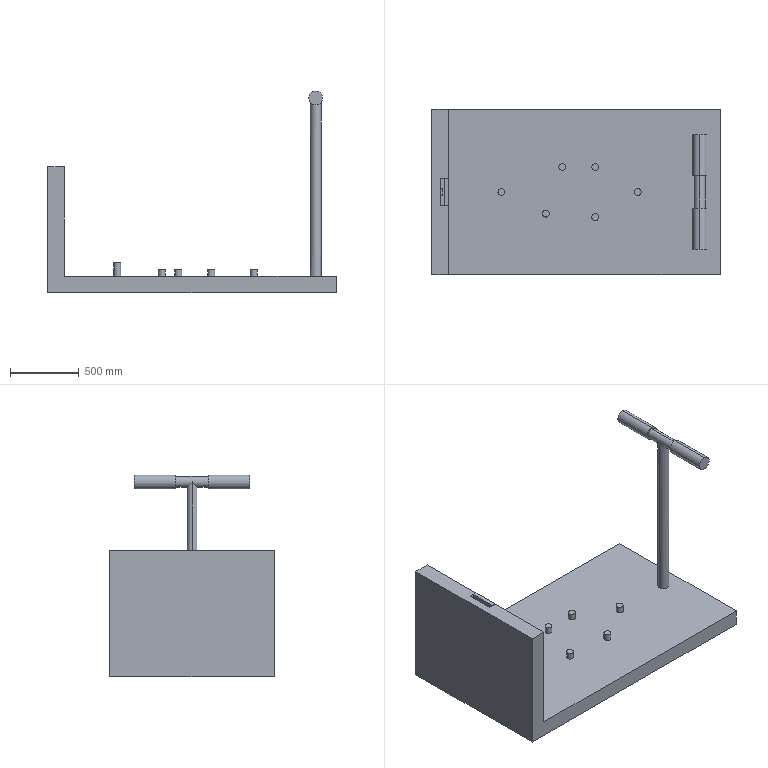Part | SolidWorks | features ICE 12, Extrusion 1, MirrorPattern 1 | 2 solids | 52 faces | box 2100 x 1200 x 1470 mm | volume 421779830 mm3 | plane 32 | cylinder 20 | commonest cylinder face diameters 50 x12 80 x4 100 x4
STEP:
#1=CARTESIAN_POINT('',(531.866,-600.,220.));
#2=VERTEX_POINT('',#1);
#3=CARTESIAN_POINT('',(481.866,-600.,220.));
#4=VERTEX_POINT('',#3);
#5=CARTESIAN_POINT('',(506.866,-600.,220.));
#6=DIRECTION('',(0.,0.,1.));
#7=DIRECTION('',(1.,0.,0.));
#8=AXIS2_PLACEMENT_3D('',#5,#6,#7);
#9=CIRCLE('',#8,25.);
#10=EDGE_CURVE('',#2,#4,#9,.T.);
#11=ORIENTED_EDGE('',*,*,#10,.F.);
#12=CARTESIAN_POINT('',(531.866,-600.,120.));
#13=VERTEX_POINT('',#12);
#14=CARTESIAN_POINT('',(531.866,-600.,220.));
#15=DIRECTION('',(0.,0.,-1.));
#16=VECTOR('',#15,1000.);
#17=LINE('',#14,#16);
#18=EDGE_CURVE('',#2,#13,#17,.T.);
#19=ORIENTED_EDGE('',*,*,#18,.T.);
#20=CARTESIAN_POINT('',(481.866,-600.,120.));
#21=VERTEX_POINT('',#20);
#22=CARTESIAN_POINT('',(506.866,-600.,120.));
#23=DIRECTION('',(0.,0.,1.));
#24=DIRECTION('',(1.,0.,0.));
#25=AXIS2_PLACEMENT_3D('',#22,#23,#24);
#26=CIRCLE('',#25,25.);
#27=EDGE_CURVE('',#13,#21,#26,.T.);
#28=ORIENTED_EDGE('',*,*,#27,.T.);
#29=CARTESIAN_POINT('',(481.866,-600.,220.));
#30=DIRECTION('',(0.,0.,-1.));
#31=VECTOR('',#30,1000.);
#32=LINE('',#29,#31);
#33=EDGE_CURVE('',#4,#21,#32,.T.);
#34=ORIENTED_EDGE('',*,*,#33,.F.);
#35=EDGE_LOOP('',(#11,#19,#28,#34));
#36=FACE_OUTER_BOUND('',#35,.T.);
#37=CARTESIAN_POINT('',(506.866,-600.,220.));
#38=DIRECTION('',(0.,0.,-1.));
#39=DIRECTION('',(-1.,0.,0.));
#40=AXIS2_PLACEMENT_3D('',#37,#38,#39);
#41=CYLINDRICAL_SURFACE('',#40,25.);
#42=ADVANCED_FACE('',(#36),#41,.T.);
#43=CARTESIAN_POINT('',(855.963,-756.72,170.));
#44=VERTEX_POINT('',#43);
#45=CARTESIAN_POINT('',(805.963,-756.72,170.));
#46=VERTEX_POINT('',#45);
#47=CARTESIAN_POINT('',(830.963,-756.72,170.));
#48=DIRECTION('',(0.,0.,1.));
#49=DIRECTION('',(1.,0.,0.));
#50=AXIS2_PLACEMENT_3D('',#47,#48,#49);
#51=CIRCLE('',#50,25.);
#52=EDGE_CURVE('',#44,#46,#51,.T.);
#53=ORIENTED_EDGE('',*,*,#52,.F.);
#54=CARTESIAN_POINT('',(855.963,-756.72,120.));
#55=VERTEX_POINT('',#54);
#56=CARTESIAN_POINT('',(855.963,-756.72,170.));
#57=DIRECTION('',(0.,0.,-1.));
#58=VECTOR('',#57,1000.);
#59=LINE('',#56,#58);
#60=EDGE_CURVE('',#44,#55,#59,.T.);
#61=ORIENTED_EDGE('',*,*,#60,.T.);
#62=CARTESIAN_POINT('',(805.963,-756.72,120.));
#63=VERTEX_POINT('',#62);
#64=CARTESIAN_POINT('',(830.963,-756.72,120.));
#65=DIRECTION('',(0.,0.,1.));
#66=DIRECTION('',(1.,0.,0.));
#67=AXIS2_PLACEMENT_3D('',#64,#65,#66);
#68=CIRCLE('',#67,25.);
#69=EDGE_CURVE('',#55,#63,#68,.T.);
#70=ORIENTED_EDGE('',*,*,#69,.T.);
#71=CARTESIAN_POINT('',(805.963,-756.72,170.));
#72=DIRECTION('',(0.,0.,-1.));
#73=VECTOR('',#72,1000.);
#74=LINE('',#71,#73);
#75=EDGE_CURVE('',#46,#63,#74,.T.);
#76=ORIENTED_EDGE('',*,*,#75,.F.);
#77=EDGE_LOOP('',(#53,#61,#70,#76));
#78=FACE_OUTER_BOUND('',#77,.T.);
#79=CARTESIAN_POINT('',(830.963,-756.72,170.));
#80=DIRECTION('',(0.,0.,-1.));
#81=DIRECTION('',(-1.,0.,0.));
#82=AXIS2_PLACEMENT_3D('',#79,#80,#81);
#83=CYLINDRICAL_SURFACE('',#82,25.);
#84=ADVANCED_FACE('',(#78),#83,.T.);
#85=CARTESIAN_POINT('',(975.,-416.97,170.));
#86=VERTEX_POINT('',#85);
#87=CARTESIAN_POINT('',(925.,-416.97,170.));
#88=VERTEX_POINT('',#87);
#89=CARTESIAN_POINT('',(950.,-416.97,170.));
#90=DIRECTION('',(0.,0.,1.));
#91=DIRECTION('',(1.,0.,0.));
#92=AXIS2_PLACEMENT_3D('',#89,#90,#91);
#93=CIRCLE('',#92,25.);
#94=EDGE_CURVE('',#86,#88,#93,.T.);
#95=ORIENTED_EDGE('',*,*,#94,.F.);
#96=CARTESIAN_POINT('',(975.,-416.97,120.));
#97=VERTEX_POINT('',#96);
#98=CARTESIAN_POINT('',(975.,-416.97,170.));
#99=DIRECTION('',(0.,0.,-1.));
#100=VECTOR('',#99,1000.);
#101=LINE('',#98,#100);
#102=EDGE_CURVE('',#86,#97,#101,.T.);
#103=ORIENTED_EDGE('',*,*,#102,.T.);
#104=CARTESIAN_POINT('',(925.,-416.97,120.));
#105=VERTEX_POINT('',#104);
#106=CARTESIAN_POINT('',(950.,-416.97,120.));
#107=DIRECTION('',(0.,0.,1.));
#108=DIRECTION('',(1.,0.,0.));
#109=AXIS2_PLACEMENT_3D('',#106,#107,#108);
#110=CIRCLE('',#109,25.);
#111=EDGE_CURVE('',#97,#105,#110,.T.);
#112=ORIENTED_EDGE('',*,*,#111,.T.);
#113=CARTESIAN_POINT('',(925.,-416.97,170.));
#114=DIRECTION('',(0.,0.,-1.));
#115=VECTOR('',#114,1000.);
#116=LINE('',#113,#115);
#117=EDGE_CURVE('',#88,#105,#116,.T.);
#118=ORIENTED_EDGE('',*,*,#117,.F.);
#119=EDGE_LOOP('',(#95,#103,#112,#118));
#120=FACE_OUTER_BOUND('',#119,.T.);
#121=CARTESIAN_POINT('',(950.,-416.97,170.));
#122=DIRECTION('',(0.,0.,-1.));
#123=DIRECTION('',(-1.,0.,0.));
#124=AXIS2_PLACEMENT_3D('',#121,#122,#123);
#125=CYLINDRICAL_SURFACE('',#124,25.);
#126=ADVANCED_FACE('',(#120),#125,.T.);
#127=CARTESIAN_POINT('',(1215.,-783.03,170.));
#128=VERTEX_POINT('',#127);
#129=CARTESIAN_POINT('',(1165.,-783.03,170.));
#130=VERTEX_POINT('',#129);
#131=CARTESIAN_POINT('',(1190.,-783.03,170.));
#132=DIRECTION('',(0.,0.,1.));
#133=DIRECTION('',(1.,0.,0.));
#134=AXIS2_PLACEMENT_3D('',#131,#132,#133);
#135=CIRCLE('',#134,25.);
#136=EDGE_CURVE('',#128,#130,#135,.T.);
#137=ORIENTED_EDGE('',*,*,#136,.F.);
#138=CARTESIAN_POINT('',(1215.,-783.03,120.));
#139=VERTEX_POINT('',#138);
#140=CARTESIAN_POINT('',(1215.,-783.03,170.));
#141=DIRECTION('',(0.,0.,-1.));
#142=VECTOR('',#141,1000.);
#143=LINE('',#140,#142);
#144=EDGE_CURVE('',#128,#139,#143,.T.);
#145=ORIENTED_EDGE('',*,*,#144,.T.);
#146=CARTESIAN_POINT('',(1165.,-783.03,120.));
#147=VERTEX_POINT('',#146);
#148=CARTESIAN_POINT('',(1190.,-783.03,120.));
#149=DIRECTION('',(0.,0.,1.));
#150=DIRECTION('',(1.,0.,0.));
#151=AXIS2_PLACEMENT_3D('',#148,#149,#150);
#152=CIRCLE('',#151,25.);
#153=EDGE_CURVE('',#139,#147,#152,.T.);
#154=ORIENTED_EDGE('',*,*,#153,.T.);
#155=CARTESIAN_POINT('',(1165.,-783.03,170.));
#156=DIRECTION('',(0.,0.,-1.));
#157=VECTOR('',#156,1000.);
#158=LINE('',#155,#157);
#159=EDGE_CURVE('',#130,#147,#158,.T.);
#160=ORIENTED_EDGE('',*,*,#159,.F.);
#161=EDGE_LOOP('',(#137,#145,#154,#160));
#162=FACE_OUTER_BOUND('',#161,.T.);
#163=CARTESIAN_POINT('',(1190.,-783.03,170.));
#164=DIRECTION('',(0.,0.,-1.));
#165=DIRECTION('',(-1.,0.,0.));
#166=AXIS2_PLACEMENT_3D('',#163,#164,#165);
#167=CYLINDRICAL_SURFACE('',#166,25.);
#168=ADVANCED_FACE('',(#162),#167,.T.);
#169=CARTESIAN_POINT('',(1215.,-416.97,170.));
#170=VERTEX_POINT('',#169);
#171=CARTESIAN_POINT('',(1165.,-416.97,170.));
#172=VERTEX_POINT('',#171);
#173=CARTESIAN_POINT('',(1190.,-416.97,170.));
#174=DIRECTION('',(0.,0.,1.));
#175=DIRECTION('',(1.,0.,0.));
#176=AXIS2_PLACEMENT_3D('',#173,#174,#175);
#177=CIRCLE('',#176,25.);
#178=EDGE_CURVE('',#170,#172,#177,.T.);
#179=ORIENTED_EDGE('',*,*,#178,.F.);
#180=CARTESIAN_POINT('',(1215.,-416.97,120.));
#181=VERTEX_POINT('',#180);
#182=CARTESIAN_POINT('',(1215.,-416.97,170.));
#183=DIRECTION('',(0.,0.,-1.));
#184=VECTOR('',#183,1000.);
#185=LINE('',#182,#184);
#186=EDGE_CURVE('',#170,#181,#185,.T.);
#187=ORIENTED_EDGE('',*,*,#186,.T.);
#188=CARTESIAN_POINT('',(1165.,-416.97,120.));
#189=VERTEX_POINT('',#188);
#190=CARTESIAN_POINT('',(1190.,-416.97,120.));
#191=DIRECTION('',(0.,0.,1.));
#192=DIRECTION('',(1.,0.,0.));
#193=AXIS2_PLACEMENT_3D('',#190,#191,#192);
#194=CIRCLE('',#193,25.);
#195=EDGE_CURVE('',#181,#189,#194,.T.);
#196=ORIENTED_EDGE('',*,*,#195,.T.);
#197=CARTESIAN_POINT('',(1165.,-416.97,170.));
#198=DIRECTION('',(0.,0.,-1.));
#199=VECTOR('',#198,1000.);
#200=LINE('',#197,#199);
#201=EDGE_CURVE('',#172,#189,#200,.T.);
#202=ORIENTED_EDGE('',*,*,#201,.F.);
#203=EDGE_LOOP('',(#179,#187,#196,#202));
#204=FACE_OUTER_BOUND('',#203,.T.);
#205=CARTESIAN_POINT('',(1190.,-416.97,170.));
#206=DIRECTION('',(0.,0.,-1.));
#207=DIRECTION('',(-1.,0.,0.));
#208=AXIS2_PLACEMENT_3D('',#205,#206,#207);
#209=CYLINDRICAL_SURFACE('',#208,25.);
#210=ADVANCED_FACE('',(#204),#209,.T.);
#211=CARTESIAN_POINT('',(1525.,-600.,170.));
#212=VERTEX_POINT('',#211);
#213=CARTESIAN_POINT('',(1475.,-600.,170.));
#214=VERTEX_POINT('',#213);
#215=CARTESIAN_POINT('',(1500.,-600.,170.));
#216=DIRECTION('',(0.,0.,1.));
#217=DIRECTION('',(1.,0.,0.));
#218=AXIS2_PLACEMENT_3D('',#215,#216,#217);
#219=CIRCLE('',#218,25.);
#220=EDGE_CURVE('',#212,#214,#219,.T.);
#221=ORIENTED_EDGE('',*,*,#220,.F.);
#222=CARTESIAN_POINT('',(1525.,-600.,120.));
#223=VERTEX_POINT('',#222);
#224=CARTESIAN_POINT('',(1525.,-600.,170.));
#225=DIRECTION('',(0.,0.,-1.));
#226=VECTOR('',#225,1000.);
#227=LINE('',#224,#226);
#228=EDGE_CURVE('',#212,#223,#227,.T.);
#229=ORIENTED_EDGE('',*,*,#228,.T.);
#230=CARTESIAN_POINT('',(1475.,-600.,120.));
#231=VERTEX_POINT('',#230);
#232=CARTESIAN_POINT('',(1500.,-600.,120.));
#233=DIRECTION('',(0.,0.,1.));
#234=DIRECTION('',(1.,0.,0.));
#235=AXIS2_PLACEMENT_3D('',#232,#233,#234);
#236=CIRCLE('',#235,25.);
#237=EDGE_CURVE('',#223,#231,#236,.T.);
#238=ORIENTED_EDGE('',*,*,#237,.T.);
#239=CARTESIAN_POINT('',(1475.,-600.,170.));
#240=DIRECTION('',(0.,0.,-1.));
#241=VECTOR('',#240,1000.);
#242=LINE('',#239,#241);
#243=EDGE_CURVE('',#214,#231,#242,.T.);
#244=ORIENTED_EDGE('',*,*,#243,.F.);
#245=EDGE_LOOP('',(#221,#229,#238,#244));
#246=FACE_OUTER_BOUND('',#245,.T.);
#247=CARTESIAN_POINT('',(1500.,-600.,170.));
#248=DIRECTION('',(0.,0.,-1.));
#249=DIRECTION('',(-1.,0.,0.));
#250=AXIS2_PLACEMENT_3D('',#247,#248,#249);
#251=CYLINDRICAL_SURFACE('',#250,25.);
#252=ADVANCED_FACE('',(#246),#251,.T.);
#253=CARTESIAN_POINT('',(1950.,-180.,1370.));
#254=VERTEX_POINT('',#253);
#255=CARTESIAN_POINT('',(1950.,-180.,1470.));
#256=VERTEX_POINT('',#255);
#257=CARTESIAN_POINT('',(1950.,-180.,1420.));
#258=DIRECTION('',(0.,-1.,0.));
#259=DIRECTION('',(0.,0.,-1.));
#260=AXIS2_PLACEMENT_3D('',#257,#258,#259);
#261=CIRCLE('',#260,50.);
#262=EDGE_CURVE('',#254,#256,#261,.T.);
#263=ORIENTED_EDGE('',*,*,#262,.T.);
#264=CARTESIAN_POINT('',(1950.,-480.,1470.));
#265=VERTEX_POINT('',#264);
#266=CARTESIAN_POINT('',(1950.,-180.,1470.));
#267=DIRECTION('',(0.,-1.,0.));
#268=VECTOR('',#267,1000.);
#269=LINE('',#266,#268);
#270=EDGE_CURVE('',#256,#265,#269,.T.);
#271=ORIENTED_EDGE('',*,*,#270,.T.);
#272=CARTESIAN_POINT('',(1950.,-480.,1370.));
#273=VERTEX_POINT('',#272);
#274=CARTESIAN_POINT('',(1950.,-480.,1420.));
#275=DIRECTION('',(0.,-1.,0.));
#276=DIRECTION('',(0.,0.,-1.));
#277=AXIS2_PLACEMENT_3D('',#274,#275,#276);
#278=CIRCLE('',#277,50.);
#279=EDGE_CURVE('',#273,#265,#278,.T.);
#280=ORIENTED_EDGE('',*,*,#279,.F.);
#281=CARTESIAN_POINT('',(1950.,-180.,1370.));
#282=DIRECTION('',(0.,-1.,0.));
#283=VECTOR('',#282,1000.);
#284=LINE('',#281,#283);
#285=EDGE_CURVE('',#254,#273,#284,.T.);
#286=ORIENTED_EDGE('',*,*,#285,.F.);
#287=EDGE_LOOP('',(#263,#271,#280,#286));
#288=FACE_OUTER_BOUND('',#287,.T.);
#289=CARTESIAN_POINT('',(1950.,-180.,1420.));
#290=DIRECTION('',(0.,-1.,0.));
#291=DIRECTION('',(0.,0.,-1.));
#292=AXIS2_PLACEMENT_3D('',#289,#290,#291);
#293=CYLINDRICAL_SURFACE('',#292,50.);
#294=ADVANCED_FACE('',(#288),#293,.T.);
#295=CARTESIAN_POINT('',(1950.,-1020.,1370.));
#296=VERTEX_POINT('',#295);
#297=CARTESIAN_POINT('',(1950.,-1020.,1470.));
#298=VERTEX_POINT('',#297);
#299=CARTESIAN_POINT('',(1950.,-1020.,1420.));
#300=DIRECTION('',(0.,-1.,0.));
#301=DIRECTION('',(0.,0.,-1.));
#302=AXIS2_PLACEMENT_3D('',#299,#300,#301);
#303=CIRCLE('',#302,50.);
#304=EDGE_CURVE('',#296,#298,#303,.T.);
#305=ORIENTED_EDGE('',*,*,#304,.F.);
#306=CARTESIAN_POINT('',(1950.,-720.,1370.));
#307=VERTEX_POINT('',#306);
#308=CARTESIAN_POINT('',(1950.,-1020.,1370.));
#309=DIRECTION('',(0.,1.,0.));
#310=VECTOR('',#309,1000.);
#311=LINE('',#308,#310);
#312=EDGE_CURVE('',#296,#307,#311,.T.);
#313=ORIENTED_EDGE('',*,*,#312,.T.);
#314=CARTESIAN_POINT('',(1950.,-720.,1470.));
#315=VERTEX_POINT('',#314);
#316=CARTESIAN_POINT('',(1950.,-720.,1420.));
#317=DIRECTION('',(0.,-1.,0.));
#318=DIRECTION('',(0.,0.,-1.));
#319=AXIS2_PLACEMENT_3D('',#316,#317,#318);
#320=CIRCLE('',#319,50.);
#321=EDGE_CURVE('',#307,#315,#320,.T.);
#322=ORIENTED_EDGE('',*,*,#321,.T.);
#323=CARTESIAN_POINT('',(1950.,-1020.,1470.));
#324=DIRECTION('',(0.,1.,0.));
#325=VECTOR('',#324,1000.);
#326=LINE('',#323,#325);
#327=EDGE_CURVE('',#298,#315,#326,.T.);
#328=ORIENTED_EDGE('',*,*,#327,.F.);
#329=EDGE_LOOP('',(#305,#313,#322,#328));
#330=FACE_OUTER_BOUND('',#329,.T.);
#331=CARTESIAN_POINT('',(1950.,-1020.,1420.));
#332=DIRECTION('',(0.,1.,0.));
#333=DIRECTION('',(0.,0.,1.));
#334=AXIS2_PLACEMENT_3D('',#331,#332,#333);
#335=CYLINDRICAL_SURFACE('',#334,50.);
#336=ADVANCED_FACE('',(#330),#335,.T.);
#337=CARTESIAN_POINT('',(1950.,-480.,1380.));
#338=VERTEX_POINT('',#337);
#339=CARTESIAN_POINT('',(1950.,-480.,1460.));
#340=VERTEX_POINT('',#339);
#341=CARTESIAN_POINT('',(1950.,-480.,1420.));
#342=DIRECTION('',(0.,-1.,0.));
#343=DIRECTION('',(0.,0.,-1.));
#344=AXIS2_PLACEMENT_3D('',#341,#342,#343);
#345=CIRCLE('',#344,40.);
#346=EDGE_CURVE('',#338,#340,#345,.T.);
#347=ORIENTED_EDGE('',*,*,#346,.T.);
#348=CARTESIAN_POINT('',(1950.,-720.,1460.));
#349=VERTEX_POINT('',#348);
#350=CARTESIAN_POINT('',(1950.,-480.,1460.));
#351=DIRECTION('',(0.,-1.,0.));
#352=VECTOR('',#351,1000.);
#353=LINE('',#350,#352);
#354=EDGE_CURVE('',#340,#349,#353,.T.);
#355=ORIENTED_EDGE('',*,*,#354,.T.);
#356=CARTESIAN_POINT('',(1950.,-720.,1380.));
#357=VERTEX_POINT('',#356);
#358=CARTESIAN_POINT('',(1950.,-720.,1420.));
#359=DIRECTION('',(0.,-1.,0.));
#360=DIRECTION('',(0.,0.,-1.));
#361=AXIS2_PLACEMENT_3D('',#358,#359,#360);
#362=CIRCLE('',#361,40.);
#363=EDGE_CURVE('',#357,#349,#362,.T.);
#364=ORIENTED_EDGE('',*,*,#363,.F.);
#365=CARTESIAN_POINT('',(1950.,-640.,1380.));
#366=VERTEX_POINT('',#365);
#367=CARTESIAN_POINT('',(1950.,-480.,1380.));
#368=DIRECTION('',(0.,-1.,0.));
#369=VECTOR('',#368,1000.);
#370=LINE('',#367,#369);
#371=EDGE_CURVE('',#366,#357,#370,.T.);
#372=ORIENTED_EDGE('',*,*,#371,.F.);
#373=CARTESIAN_POINT('',(1990.,-600.,1420.));
#374=VERTEX_POINT('',#373);
#375=CARTESIAN_POINT('',(1990.,-600.,1420.));
#376=CARTESIAN_POINT('',(1990.,-623.431,1396.569));
#377=CARTESIAN_POINT('',(1973.431,-640.,1380.));
#378=CARTESIAN_POINT('',(1950.,-640.,1380.));
#379=(BOUNDED_CURVE()B_SPLINE_CURVE(3,(#375,#376,#377,#378),.UNSPECIFIED.,.F.,.F.)B_SPLINE_CURVE_WITH_KNOTS((4,4),(4.712,6.283),.UNSPECIFIED.)CURVE()GEOMETRIC_REPRESENTATION_ITEM()RATIONAL_B_SPLINE_CURVE((1.,0.8047,0.8047,1.))REPRESENTATION_ITEM(''));
#380=EDGE_CURVE('',#374,#366,#379,.T.);
#381=ORIENTED_EDGE('',*,*,#380,.F.);
#382=CARTESIAN_POINT('',(1950.,-560.,1380.));
#383=VERTEX_POINT('',#382);
#384=CARTESIAN_POINT('',(1950.,-560.,1380.));
#385=CARTESIAN_POINT('',(1973.431,-560.,1380.));
#386=CARTESIAN_POINT('',(1990.,-576.569,1396.569));
#387=CARTESIAN_POINT('',(1990.,-600.,1420.));
#388=(BOUNDED_CURVE()B_SPLINE_CURVE(3,(#384,#385,#386,#387),.UNSPECIFIED.,.F.,.F.)B_SPLINE_CURVE_WITH_KNOTS((4,4),(0.,1.571),.UNSPECIFIED.)CURVE()GEOMETRIC_REPRESENTATION_ITEM()RATIONAL_B_SPLINE_CURVE((1.,0.8047,0.8047,1.))REPRESENTATION_ITEM(''));
#389=EDGE_CURVE('',#383,#374,#388,.T.);
#390=ORIENTED_EDGE('',*,*,#389,.F.);
#391=CARTESIAN_POINT('',(1950.,-480.,1380.));
#392=DIRECTION('',(0.,-1.,0.));
#393=VECTOR('',#392,1000.);
#394=LINE('',#391,#393);
#395=EDGE_CURVE('',#338,#383,#394,.T.);
#396=ORIENTED_EDGE('',*,*,#395,.F.);
#397=EDGE_LOOP('',(#347,#355,#364,#372,#381,#390,#396));
#398=FACE_OUTER_BOUND('',#397,.T.);
#399=CARTESIAN_POINT('',(1950.,-480.,1420.));
#400=DIRECTION('',(0.,-1.,0.));
#401=DIRECTION('',(0.,0.,-1.));
#402=AXIS2_PLACEMENT_3D('',#399,#400,#401);
#403=CYLINDRICAL_SURFACE('',#402,40.);
#404=ADVANCED_FACE('',(#398),#403,.T.);
#405=CARTESIAN_POINT('',(1910.,-600.,1420.));
#406=VERTEX_POINT('',#405);
#407=CARTESIAN_POINT('',(1910.,-600.,1420.));
#408=CARTESIAN_POINT('',(1910.,-576.569,1396.569));
#409=CARTESIAN_POINT('',(1926.569,-560.,1380.));
#410=CARTESIAN_POINT('',(1950.,-560.,1380.));
#411=(BOUNDED_CURVE()B_SPLINE_CURVE(3,(#407,#408,#409,#410),.UNSPECIFIED.,.F.,.F.)B_SPLINE_CURVE_WITH_KNOTS((4,4),(4.712,6.283),.UNSPECIFIED.)CURVE()GEOMETRIC_REPRESENTATION_ITEM()RATIONAL_B_SPLINE_CURVE((1.,0.8047,0.8047,1.))REPRESENTATION_ITEM(''));
#412=EDGE_CURVE('',#406,#383,#411,.T.);
#413=ORIENTED_EDGE('',*,*,#412,.T.);
#414=ORIENTED_EDGE('',*,*,#389,.T.);
#415=CARTESIAN_POINT('',(1990.,-600.,120.));
#416=VERTEX_POINT('',#415);
#417=CARTESIAN_POINT('',(1990.,-600.,1420.));
#418=DIRECTION('',(0.,0.,-1.));
#419=VECTOR('',#418,1000.);
#420=LINE('',#417,#419);
#421=EDGE_CURVE('',#374,#416,#420,.T.);
#422=ORIENTED_EDGE('',*,*,#421,.T.);
#423=CARTESIAN_POINT('',(1910.,-600.,120.));
#424=VERTEX_POINT('',#423);
#425=CARTESIAN_POINT('',(1950.,-600.,120.));
#426=DIRECTION('',(0.,0.,1.));
#427=DIRECTION('',(1.,0.,0.));
#428=AXIS2_PLACEMENT_3D('',#425,#426,#427);
#429=CIRCLE('',#428,40.);
#430=EDGE_CURVE('',#416,#424,#429,.T.);
#431=ORIENTED_EDGE('',*,*,#430,.T.);
#432=CARTESIAN_POINT('',(1910.,-600.,1420.));
#433=DIRECTION('',(0.,0.,-1.));
#434=VECTOR('',#433,1000.);
#435=LINE('',#432,#434);
#436=EDGE_CURVE('',#406,#424,#435,.T.);
#437=ORIENTED_EDGE('',*,*,#436,.F.);
#438=EDGE_LOOP('',(#413,#414,#422,#431,#437));
#439=FACE_OUTER_BOUND('',#438,.T.);
#440=CARTESIAN_POINT('',(1950.,-600.,1420.));
#441=DIRECTION('',(0.,0.,-1.));
#442=DIRECTION('',(-1.,0.,0.));
#443=AXIS2_PLACEMENT_3D('',#440,#441,#442);
#444=CYLINDRICAL_SURFACE('',#443,40.);
#445=ADVANCED_FACE('',(#439),#444,.T.);
#446=CARTESIAN_POINT('',(506.866,-600.,120.));
#447=DIRECTION('',(0.,0.,1.));
#448=DIRECTION('',(1.,0.,0.));
#449=AXIS2_PLACEMENT_3D('',#446,#447,#448);
#450=CIRCLE('',#449,25.);
#451=EDGE_CURVE('',#21,#13,#450,.T.);
#452=ORIENTED_EDGE('',*,*,#451,.F.);
#453=ORIENTED_EDGE('',*,*,#27,.F.);
#454=EDGE_LOOP('',(#452,#453));
#455=FACE_BOUND('',#454,.T.);
#456=CARTESIAN_POINT('',(830.963,-756.72,120.));
#457=DIRECTION('',(0.,0.,1.));
#458=DIRECTION('',(1.,0.,0.));
#459=AXIS2_PLACEMENT_3D('',#456,#457,#458);
#460=CIRCLE('',#459,25.);
#461=EDGE_CURVE('',#63,#55,#460,.T.);
#462=ORIENTED_EDGE('',*,*,#461,.F.);
#463=ORIENTED_EDGE('',*,*,#69,.F.);
#464=EDGE_LOOP('',(#462,#463));
#465=FACE_BOUND('',#464,.T.);
#466=CARTESIAN_POINT('',(950.,-416.97,120.));
#467=DIRECTION('',(0.,0.,1.));
#468=DIRECTION('',(1.,0.,0.));
#469=AXIS2_PLACEMENT_3D('',#466,#467,#468);
#470=CIRCLE('',#469,25.);
#471=EDGE_CURVE('',#105,#97,#470,.T.);
#472=ORIENTED_EDGE('',*,*,#471,.F.);
#473=ORIENTED_EDGE('',*,*,#111,.F.);
#474=EDGE_LOOP('',(#472,#473));
#475=FACE_BOUND('',#474,.T.);
#476=CARTESIAN_POINT('',(1190.,-783.03,120.));
#477=DIRECTION('',(0.,0.,1.));
#478=DIRECTION('',(1.,0.,0.));
#479=AXIS2_PLACEMENT_3D('',#476,#477,#478);
#480=CIRCLE('',#479,25.);
#481=EDGE_CURVE('',#147,#139,#480,.T.);
#482=ORIENTED_EDGE('',*,*,#481,.F.);
#483=ORIENTED_EDGE('',*,*,#153,.F.);
#484=EDGE_LOOP('',(#482,#483));
#485=FACE_BOUND('',#484,.T.);
#486=CARTESIAN_POINT('',(1190.,-416.97,120.));
#487=DIRECTION('',(0.,0.,1.));
#488=DIRECTION('',(1.,0.,0.));
#489=AXIS2_PLACEMENT_3D('',#486,#487,#488);
#490=CIRCLE('',#489,25.);
#491=EDGE_CURVE('',#189,#181,#490,.T.);
#492=ORIENTED_EDGE('',*,*,#491,.F.);
#493=ORIENTED_EDGE('',*,*,#195,.F.);
#494=EDGE_LOOP('',(#492,#493));
#495=FACE_BOUND('',#494,.T.);
#496=CARTESIAN_POINT('',(1500.,-600.,120.));
#497=DIRECTION('',(0.,0.,1.));
#498=DIRECTION('',(1.,0.,0.));
#499=AXIS2_PLACEMENT_3D('',#496,#497,#498);
#500=CIRCLE('',#499,25.);
#501=EDGE_CURVE('',#231,#223,#500,.T.);
#502=ORIENTED_EDGE('',*,*,#501,.F.);
#503=ORIENTED_EDGE('',*,*,#237,.F.);
#504=EDGE_LOOP('',(#502,#503));
#505=FACE_BOUND('',#504,.T.);
#506=CARTESIAN_POINT('',(1950.,-600.,120.));
#507=DIRECTION('',(0.,0.,1.));
#508=DIRECTION('',(1.,0.,0.));
#509=AXIS2_PLACEMENT_3D('',#506,#507,#508);
#510=CIRCLE('',#509,40.);
#511=EDGE_CURVE('',#424,#416,#510,.T.);
#512=ORIENTED_EDGE('',*,*,#511,.F.);
#513=ORIENTED_EDGE('',*,*,#430,.F.);
#514=EDGE_LOOP('',(#512,#513));
#515=FACE_BOUND('',#514,.T.);
#516=CARTESIAN_POINT('',(80.,-625.,120.));
#517=VERTEX_POINT('',#516);
#518=CARTESIAN_POINT('',(80.,-575.,120.));
#519=VERTEX_POINT('',#518);
#520=CARTESIAN_POINT('',(80.,-575.,120.));
#521=DIRECTION('',(0.,1.,0.));
#522=VECTOR('',#521,1000.);
#523=LINE('',#520,#522);
#524=EDGE_CURVE('',#517,#519,#523,.T.);
#525=ORIENTED_EDGE('',*,*,#524,.F.);
#526=CARTESIAN_POINT('',(60.,-625.,120.));
#527=VERTEX_POINT('',#526);
#528=CARTESIAN_POINT('',(80.,-625.,120.));
#529=DIRECTION('',(-1.,0.,0.));
#530=VECTOR('',#529,1000.);
#531=LINE('',#528,#530);
#532=EDGE_CURVE('',#517,#527,#531,.T.);
#533=ORIENTED_EDGE('',*,*,#532,.T.);
#534=CARTESIAN_POINT('',(60.,-700.,120.));
#535=VERTEX_POINT('',#534);
#536=CARTESIAN_POINT('',(60.,-500.,120.));
#537=DIRECTION('',(0.,1.,0.));
#538=VECTOR('',#537,1000.);
#539=LINE('',#536,#538);
#540=EDGE_CURVE('',#535,#527,#539,.T.);
#541=ORIENTED_EDGE('',*,*,#540,.F.);
#542=CARTESIAN_POINT('',(120.,-700.,120.));
#543=VERTEX_POINT('',#542);
#544=CARTESIAN_POINT('',(180.,-700.,120.));
#545=DIRECTION('',(-1.,0.,0.));
#546=VECTOR('',#545,1000.);
#547=LINE('',#544,#546);
#548=EDGE_CURVE('',#543,#535,#547,.T.);
#549=ORIENTED_EDGE('',*,*,#548,.F.);
#550=CARTESIAN_POINT('',(120.,-1200.,120.));
#551=VERTEX_POINT('',#550);
#552=CARTESIAN_POINT('',(120.,0.,120.));
#553=DIRECTION('',(0.,1.,0.));
#554=VECTOR('',#553,1000.);
#555=LINE('',#552,#554);
#556=EDGE_CURVE('',#551,#543,#555,.T.);
#557=ORIENTED_EDGE('',*,*,#556,.F.);
#558=CARTESIAN_POINT('',(2100.,-1200.,120.));
#559=VERTEX_POINT('',#558);
#560=CARTESIAN_POINT('',(0.,-1200.,120.));
#561=DIRECTION('',(1.,0.,0.));
#562=VECTOR('',#561,1000.);
#563=LINE('',#560,#562);
#564=EDGE_CURVE('',#551,#559,#563,.T.);
#565=ORIENTED_EDGE('',*,*,#564,.T.);
#566=CARTESIAN_POINT('',(2100.,0.,120.));
#567=VERTEX_POINT('',#566);
#568=CARTESIAN_POINT('',(2100.,0.,120.));
#569=DIRECTION('',(0.,1.,0.));
#570=VECTOR('',#569,1000.);
#571=LINE('',#568,#570);
#572=EDGE_CURVE('',#559,#567,#571,.T.);
#573=ORIENTED_EDGE('',*,*,#572,.T.);
#574=CARTESIAN_POINT('',(120.,0.,120.));
#575=VERTEX_POINT('',#574);
#576=CARTESIAN_POINT('',(0.,0.,120.));
#577=DIRECTION('',(-1.,0.,0.));
#578=VECTOR('',#577,1000.);
#579=LINE('',#576,#578);
#580=EDGE_CURVE('',#567,#575,#579,.T.);
#581=ORIENTED_EDGE('',*,*,#580,.T.);
#582=CARTESIAN_POINT('',(120.,-500.,120.));
#583=VERTEX_POINT('',#582);
#584=CARTESIAN_POINT('',(120.,0.,120.));
#585=DIRECTION('',(0.,1.,0.));
#586=VECTOR('',#585,1000.);
#587=LINE('',#584,#586);
#588=EDGE_CURVE('',#583,#575,#587,.T.);
#589=ORIENTED_EDGE('',*,*,#588,.F.);
#590=CARTESIAN_POINT('',(60.,-500.,120.));
#591=VERTEX_POINT('',#590);
#592=CARTESIAN_POINT('',(180.,-500.,120.));
#593=DIRECTION('',(1.,0.,0.));
#594=VECTOR('',#593,1000.);
#595=LINE('',#592,#594);
#596=EDGE_CURVE('',#591,#583,#595,.T.);
#597=ORIENTED_EDGE('',*,*,#596,.F.);
#598=CARTESIAN_POINT('',(60.,-575.,120.));
#599=VERTEX_POINT('',#598);
#600=CARTESIAN_POINT('',(60.,-500.,120.));
#601=DIRECTION('',(0.,1.,0.));
#602=VECTOR('',#601,1000.);
#603=LINE('',#600,#602);
#604=EDGE_CURVE('',#599,#591,#603,.T.);
#605=ORIENTED_EDGE('',*,*,#604,.F.);
#606=CARTESIAN_POINT('',(80.,-575.,120.));
#607=DIRECTION('',(-1.,0.,0.));
#608=VECTOR('',#607,1000.);
#609=LINE('',#606,#608);
#610=EDGE_CURVE('',#519,#599,#609,.T.);
#611=ORIENTED_EDGE('',*,*,#610,.F.);
#612=EDGE_LOOP('',(#525,#533,#541,#549,#557,#565,#573,#581,#589,#597,#605,#611));
#613=FACE_OUTER_BOUND('',#612,.T.);
#614=CARTESIAN_POINT('',(0.,0.,120.));
#615=DIRECTION('',(0.,0.,1.));
#616=DIRECTION('',(1.,0.,0.));
#617=AXIS2_PLACEMENT_3D('',#614,#615,#616);
#618=PLANE('',#617);
#619=ADVANCED_FACE('',(#455,#465,#475,#485,#495,#505,#515,#613),#618,.T.);
#620=CARTESIAN_POINT('',(60.,-625.,630.));
#621=VERTEX_POINT('',#620);
#622=CARTESIAN_POINT('',(60.,-625.,120.));
#623=DIRECTION('',(0.,0.,-1.));
#624=VECTOR('',#623,1000.);
#625=LINE('',#622,#624);
#626=EDGE_CURVE('',#621,#527,#625,.T.);
#627=ORIENTED_EDGE('',*,*,#626,.F.);
#628=CARTESIAN_POINT('',(60.,-575.,630.));
#629=VERTEX_POINT('',#628);
#630=CARTESIAN_POINT('',(60.,-575.,630.));
#631=DIRECTION('',(0.,-1.,0.));
#632=VECTOR('',#631,1000.);
#633=LINE('',#630,#632);
#634=EDGE_CURVE('',#629,#621,#633,.T.);
#635=ORIENTED_EDGE('',*,*,#634,.F.);
#636=CARTESIAN_POINT('',(60.,-575.,120.));
#637=DIRECTION('',(0.,0.,1.));
#638=VECTOR('',#637,1000.);
#639=LINE('',#636,#638);
#640=EDGE_CURVE('',#599,#629,#639,.T.);
#641=ORIENTED_EDGE('',*,*,#640,.F.);
#642=ORIENTED_EDGE('',*,*,#604,.T.);
#643=CARTESIAN_POINT('',(60.,-500.,920.));
#644=VERTEX_POINT('',#643);
#645=CARTESIAN_POINT('',(60.,-500.,-113.238));
#646=DIRECTION('',(0.,0.,1.));
#647=VECTOR('',#646,1000.);
#648=LINE('',#645,#647);
#649=EDGE_CURVE('',#591,#644,#648,.T.);
#650=ORIENTED_EDGE('',*,*,#649,.T.);
#651=CARTESIAN_POINT('',(60.,-700.,920.));
#652=VERTEX_POINT('',#651);
#653=CARTESIAN_POINT('',(60.,-500.,920.));
#654=DIRECTION('',(0.,-1.,0.));
#655=VECTOR('',#654,1000.);
#656=LINE('',#653,#655);
#657=EDGE_CURVE('',#644,#652,#656,.T.);
#658=ORIENTED_EDGE('',*,*,#657,.T.);
#659=CARTESIAN_POINT('',(60.,-700.,-113.238));
#660=DIRECTION('',(0.,0.,1.));
#661=VECTOR('',#660,1000.);
#662=LINE('',#659,#661);
#663=EDGE_CURVE('',#535,#652,#662,.T.);
#664=ORIENTED_EDGE('',*,*,#663,.F.);
#665=ORIENTED_EDGE('',*,*,#540,.T.);
#666=EDGE_LOOP('',(#627,#635,#641,#642,#650,#658,#664,#665));
#667=FACE_OUTER_BOUND('',#666,.T.);
#668=CARTESIAN_POINT('',(60.,-500.,-113.238));
#669=DIRECTION('',(-1.,0.,0.));
#670=DIRECTION('',(0.,-1.,0.));
#671=AXIS2_PLACEMENT_3D('',#668,#669,#670);
#672=PLANE('',#671);
#673=ADVANCED_FACE('',(#667),#672,.F.);
#674=CARTESIAN_POINT('',(120.,-500.,920.));
#675=VERTEX_POINT('',#674);
#676=CARTESIAN_POINT('',(120.,0.,920.));
#677=VERTEX_POINT('',#676);
#678=CARTESIAN_POINT('',(120.,0.,920.));
#679=DIRECTION('',(0.,1.,0.));
#680=VECTOR('',#679,1000.);
#681=LINE('',#678,#680);
#682=EDGE_CURVE('',#675,#677,#681,.T.);
#683=ORIENTED_EDGE('',*,*,#682,.F.);
#684=CARTESIAN_POINT('',(120.,-500.,920.));
#685=DIRECTION('',(0.,0.,-1.));
#686=VECTOR('',#685,1000.);
#687=LINE('',#684,#686);
#688=EDGE_CURVE('',#675,#583,#687,.T.);
#689=ORIENTED_EDGE('',*,*,#688,.T.);
#690=ORIENTED_EDGE('',*,*,#588,.T.);
#691=CARTESIAN_POINT('',(120.,0.,920.));
#692=DIRECTION('',(0.,0.,-1.));
#693=VECTOR('',#692,1000.);
#694=LINE('',#691,#693);
#695=EDGE_CURVE('',#677,#575,#694,.T.);
#696=ORIENTED_EDGE('',*,*,#695,.F.);
#697=EDGE_LOOP('',(#683,#689,#690,#696));
#698=FACE_OUTER_BOUND('',#697,.T.);
#699=CARTESIAN_POINT('',(120.,0.,920.));
#700=DIRECTION('',(-1.,0.,0.));
#701=DIRECTION('',(0.,-1.,0.));
#702=AXIS2_PLACEMENT_3D('',#699,#700,#701);
#703=PLANE('',#702);
#704=ADVANCED_FACE('',(#698),#703,.F.);
#705=CARTESIAN_POINT('',(0.,0.,0.));
#706=VERTEX_POINT('',#705);
#707=CARTESIAN_POINT('',(0.,-1200.,0.));
#708=VERTEX_POINT('',#707);
#709=CARTESIAN_POINT('',(0.,0.,0.));
#710=DIRECTION('',(0.,-1.,0.));
#711=VECTOR('',#710,1000.);
#712=LINE('',#709,#711);
#713=EDGE_CURVE('',#706,#708,#712,.T.);
#714=ORIENTED_EDGE('',*,*,#713,.T.);
#715=CARTESIAN_POINT('',(0.,-1200.,920.));
#716=VERTEX_POINT('',#715);
#717=CARTESIAN_POINT('',(0.,-1200.,120.));
#718=DIRECTION('',(0.,0.,-1.));
#719=VECTOR('',#718,1000.);
#720=LINE('',#717,#719);
#721=EDGE_CURVE('',#716,#708,#720,.T.);
#722=ORIENTED_EDGE('',*,*,#721,.F.);
#723=CARTESIAN_POINT('',(0.,0.,920.));
#724=VERTEX_POINT('',#723);
#725=CARTESIAN_POINT('',(0.,0.,920.));
#726=DIRECTION('',(0.,-1.,0.));
#727=VECTOR('',#726,1000.);
#728=LINE('',#725,#727);
#729=EDGE_CURVE('',#724,#716,#728,.T.);
#730=ORIENTED_EDGE('',*,*,#729,.F.);
#731=CARTESIAN_POINT('',(0.,0.,120.));
#732=DIRECTION('',(0.,0.,-1.));
#733=VECTOR('',#732,1000.);
#734=LINE('',#731,#733);
#735=EDGE_CURVE('',#724,#706,#734,.T.);
#736=ORIENTED_EDGE('',*,*,#735,.T.);
#737=EDGE_LOOP('',(#714,#722,#730,#736));
#738=FACE_OUTER_BOUND('',#737,.T.);
#739=CARTESIAN_POINT('',(0.,0.,120.));
#740=DIRECTION('',(1.,0.,0.));
#741=DIRECTION('',(0.,1.,0.));
#742=AXIS2_PLACEMENT_3D('',#739,#740,#741);
#743=PLANE('',#742);
#744=ADVANCED_FACE('',(#738),#743,.F.);
#745=CARTESIAN_POINT('',(2100.,-1200.,0.));
#746=VERTEX_POINT('',#745);
#747=CARTESIAN_POINT('',(0.,-1200.,0.));
#748=DIRECTION('',(1.,0.,0.));
#749=VECTOR('',#748,1000.);
#750=LINE('',#747,#749);
#751=EDGE_CURVE('',#708,#746,#750,.T.);
#752=ORIENTED_EDGE('',*,*,#751,.T.);
#753=CARTESIAN_POINT('',(2100.,-1200.,120.));
#754=DIRECTION('',(0.,0.,-1.));
#755=VECTOR('',#754,1000.);
#756=LINE('',#753,#755);
#757=EDGE_CURVE('',#559,#746,#756,.T.);
#758=ORIENTED_EDGE('',*,*,#757,.F.);
#759=ORIENTED_EDGE('',*,*,#564,.F.);
#760=CARTESIAN_POINT('',(120.,-1200.,920.));
#761=VERTEX_POINT('',#760);
#762=CARTESIAN_POINT('',(120.,-1200.,920.));
#763=DIRECTION('',(0.,0.,-1.));
#764=VECTOR('',#763,1000.);
#765=LINE('',#762,#764);
#766=EDGE_CURVE('',#761,#551,#765,.T.);
#767=ORIENTED_EDGE('',*,*,#766,.F.);
#768=CARTESIAN_POINT('',(0.,-1200.,920.));
#769=DIRECTION('',(1.,0.,0.));
#770=VECTOR('',#769,1000.);
#771=LINE('',#768,#770);
#772=EDGE_CURVE('',#716,#761,#771,.T.);
#773=ORIENTED_EDGE('',*,*,#772,.F.);
#774=ORIENTED_EDGE('',*,*,#721,.T.);
#775=EDGE_LOOP('',(#752,#758,#759,#767,#773,#774));
#776=FACE_OUTER_BOUND('',#775,.T.);
#777=CARTESIAN_POINT('',(0.,-1200.,120.));
#778=DIRECTION('',(0.,1.,0.));
#779=DIRECTION('',(-1.,0.,0.));
#780=AXIS2_PLACEMENT_3D('',#777,#778,#779);
#781=PLANE('',#780);
#782=ADVANCED_FACE('',(#776),#781,.F.);
#783=CARTESIAN_POINT('',(2100.,0.,0.));
#784=VERTEX_POINT('',#783);
#785=CARTESIAN_POINT('',(2100.,0.,0.));
#786=DIRECTION('',(0.,1.,0.));
#787=VECTOR('',#786,1000.);
#788=LINE('',#785,#787);
#789=EDGE_CURVE('',#746,#784,#788,.T.);
#790=ORIENTED_EDGE('',*,*,#789,.T.);
#791=CARTESIAN_POINT('',(2100.,0.,120.));
#792=DIRECTION('',(0.,0.,-1.));
#793=VECTOR('',#792,1000.);
#794=LINE('',#791,#793);
#795=EDGE_CURVE('',#567,#784,#794,.T.);
#796=ORIENTED_EDGE('',*,*,#795,.F.);
#797=ORIENTED_EDGE('',*,*,#572,.F.);
#798=ORIENTED_EDGE('',*,*,#757,.T.);
#799=EDGE_LOOP('',(#790,#796,#797,#798));
#800=FACE_OUTER_BOUND('',#799,.T.);
#801=CARTESIAN_POINT('',(2100.,0.,120.));
#802=DIRECTION('',(-1.,0.,0.));
#803=DIRECTION('',(0.,0.,1.));
#804=AXIS2_PLACEMENT_3D('',#801,#802,#803);
#805=PLANE('',#804);
#806=ADVANCED_FACE('',(#800),#805,.F.);
#807=CARTESIAN_POINT('',(0.,0.,0.));
#808=DIRECTION('',(-1.,0.,0.));
#809=VECTOR('',#808,1000.);
#810=LINE('',#807,#809);
#811=EDGE_CURVE('',#784,#706,#810,.T.);
#812=ORIENTED_EDGE('',*,*,#811,.T.);
#813=ORIENTED_EDGE('',*,*,#735,.F.);
#814=CARTESIAN_POINT('',(0.,0.,920.));
#815=DIRECTION('',(-1.,0.,0.));
#816=VECTOR('',#815,1000.);
#817=LINE('',#814,#816);
#818=EDGE_CURVE('',#677,#724,#817,.T.);
#819=ORIENTED_EDGE('',*,*,#818,.F.);
#820=ORIENTED_EDGE('',*,*,#695,.T.);
#821=ORIENTED_EDGE('',*,*,#580,.F.);
#822=ORIENTED_EDGE('',*,*,#795,.T.);
#823=EDGE_LOOP('',(#812,#813,#819,#820,#821,#822));
#824=FACE_OUTER_BOUND('',#823,.T.);
#825=CARTESIAN_POINT('',(0.,0.,120.));
#826=DIRECTION('',(0.,-1.,0.));
#827=DIRECTION('',(1.,0.,0.));
#828=AXIS2_PLACEMENT_3D('',#825,#826,#827);
#829=PLANE('',#828);
#830=ADVANCED_FACE('',(#824),#829,.F.);
#831=ORIENTED_EDGE('',*,*,#713,.F.);
#832=ORIENTED_EDGE('',*,*,#811,.F.);
#833=ORIENTED_EDGE('',*,*,#789,.F.);
#834=ORIENTED_EDGE('',*,*,#751,.F.);
#835=EDGE_LOOP('',(#831,#832,#833,#834));
#836=FACE_OUTER_BOUND('',#835,.T.);
#837=CARTESIAN_POINT('',(0.,0.,0.));
#838=DIRECTION('',(0.,0.,1.));
#839=DIRECTION('',(1.,0.,0.));
#840=AXIS2_PLACEMENT_3D('',#837,#838,#839);
#841=PLANE('',#840);
#842=ADVANCED_FACE('',(#836),#841,.F.);
#843=ORIENTED_EDGE('',*,*,#556,.T.);
#844=CARTESIAN_POINT('',(120.,-700.,920.));
#845=VERTEX_POINT('',#844);
#846=CARTESIAN_POINT('',(120.,-700.,920.));
#847=DIRECTION('',(0.,0.,1.));
#848=VECTOR('',#847,1000.);
#849=LINE('',#846,#848);
#850=EDGE_CURVE('',#543,#845,#849,.T.);
#851=ORIENTED_EDGE('',*,*,#850,.T.);
#852=CARTESIAN_POINT('',(120.,0.,920.));
#853=DIRECTION('',(0.,1.,0.));
#854=VECTOR('',#853,1000.);
#855=LINE('',#852,#854);
#856=EDGE_CURVE('',#761,#845,#855,.T.);
#857=ORIENTED_EDGE('',*,*,#856,.F.);
#858=ORIENTED_EDGE('',*,*,#766,.T.);
#859=EDGE_LOOP('',(#843,#851,#857,#858));
#860=FACE_OUTER_BOUND('',#859,.T.);
#861=CARTESIAN_POINT('',(120.,0.,920.));
#862=DIRECTION('',(-1.,0.,0.));
#863=DIRECTION('',(0.,-1.,0.));
#864=AXIS2_PLACEMENT_3D('',#861,#862,#863);
#865=PLANE('',#864);
#866=ADVANCED_FACE('',(#860),#865,.F.);
#867=CARTESIAN_POINT('',(0.,-500.,920.));
#868=DIRECTION('',(-1.,0.,0.));
#869=VECTOR('',#868,1000.);
#870=LINE('',#867,#869);
#871=EDGE_CURVE('',#675,#644,#870,.T.);
#872=ORIENTED_EDGE('',*,*,#871,.F.);
#873=ORIENTED_EDGE('',*,*,#682,.T.);
#874=ORIENTED_EDGE('',*,*,#818,.T.);
#875=ORIENTED_EDGE('',*,*,#729,.T.);
#876=ORIENTED_EDGE('',*,*,#772,.T.);
#877=ORIENTED_EDGE('',*,*,#856,.T.);
#878=CARTESIAN_POINT('',(180.,-700.,920.));
#879=DIRECTION('',(1.,0.,0.));
#880=VECTOR('',#879,1000.);
#881=LINE('',#878,#880);
#882=EDGE_CURVE('',#652,#845,#881,.T.);
#883=ORIENTED_EDGE('',*,*,#882,.F.);
#884=ORIENTED_EDGE('',*,*,#657,.F.);
#885=EDGE_LOOP('',(#872,#873,#874,#875,#876,#877,#883,#884));
#886=FACE_OUTER_BOUND('',#885,.T.);
#887=CARTESIAN_POINT('',(0.,0.,920.));
#888=DIRECTION('',(0.,0.,1.));
#889=DIRECTION('',(1.,0.,0.));
#890=AXIS2_PLACEMENT_3D('',#887,#888,#889);
#891=PLANE('',#890);
#892=ADVANCED_FACE('',(#886),#891,.T.);
#893=ORIENTED_EDGE('',*,*,#421,.F.);
#894=ORIENTED_EDGE('',*,*,#380,.T.);
#895=CARTESIAN_POINT('',(1950.,-640.,1380.));
#896=CARTESIAN_POINT('',(1926.569,-640.,1380.));
#897=CARTESIAN_POINT('',(1910.,-623.431,1396.569));
#898=CARTESIAN_POINT('',(1910.,-600.,1420.));
#899=(BOUNDED_CURVE()B_SPLINE_CURVE(3,(#895,#896,#897,#898),.UNSPECIFIED.,.F.,.F.)B_SPLINE_CURVE_WITH_KNOTS((4,4),(0.,1.571),.UNSPECIFIED.)CURVE()GEOMETRIC_REPRESENTATION_ITEM()RATIONAL_B_SPLINE_CURVE((1.,0.8047,0.8047,1.))REPRESENTATION_ITEM(''));
#900=EDGE_CURVE('',#366,#406,#899,.T.);
#901=ORIENTED_EDGE('',*,*,#900,.T.);
#902=ORIENTED_EDGE('',*,*,#436,.T.);
#903=ORIENTED_EDGE('',*,*,#511,.T.);
#904=EDGE_LOOP('',(#893,#894,#901,#902,#903));
#905=FACE_OUTER_BOUND('',#904,.T.);
#906=CARTESIAN_POINT('',(1950.,-600.,1420.));
#907=DIRECTION('',(0.,0.,-1.));
#908=DIRECTION('',(-1.,0.,0.));
#909=AXIS2_PLACEMENT_3D('',#906,#907,#908);
#910=CYLINDRICAL_SURFACE('',#909,40.);
#911=ADVANCED_FACE('',(#905),#910,.T.);
#912=ORIENTED_EDGE('',*,*,#354,.F.);
#913=CARTESIAN_POINT('',(1950.,-480.,1420.));
#914=DIRECTION('',(0.,-1.,0.));
#915=DIRECTION('',(0.,0.,-1.));
#916=AXIS2_PLACEMENT_3D('',#913,#914,#915);
#917=CIRCLE('',#916,40.);
#918=EDGE_CURVE('',#340,#338,#917,.T.);
#919=ORIENTED_EDGE('',*,*,#918,.T.);
#920=ORIENTED_EDGE('',*,*,#395,.T.);
#921=ORIENTED_EDGE('',*,*,#412,.F.);
#922=ORIENTED_EDGE('',*,*,#900,.F.);
#923=ORIENTED_EDGE('',*,*,#371,.T.);
#924=CARTESIAN_POINT('',(1950.,-720.,1420.));
#925=DIRECTION('',(0.,-1.,0.));
#926=DIRECTION('',(0.,0.,-1.));
#927=AXIS2_PLACEMENT_3D('',#924,#925,#926);
#928=CIRCLE('',#927,40.);
#929=EDGE_CURVE('',#349,#357,#928,.T.);
#930=ORIENTED_EDGE('',*,*,#929,.F.);
#931=EDGE_LOOP('',(#912,#919,#920,#921,#922,#923,#930));
#932=FACE_OUTER_BOUND('',#931,.T.);
#933=CARTESIAN_POINT('',(1950.,-480.,1420.));
#934=DIRECTION('',(0.,-1.,0.));
#935=DIRECTION('',(0.,0.,-1.));
#936=AXIS2_PLACEMENT_3D('',#933,#934,#935);
#937=CYLINDRICAL_SURFACE('',#936,40.);
#938=ADVANCED_FACE('',(#932),#937,.T.);
#939=ORIENTED_EDGE('',*,*,#312,.F.);
#940=CARTESIAN_POINT('',(1950.,-1020.,1420.));
#941=DIRECTION('',(0.,-1.,0.));
#942=DIRECTION('',(0.,0.,-1.));
#943=AXIS2_PLACEMENT_3D('',#940,#941,#942);
#944=CIRCLE('',#943,50.);
#945=EDGE_CURVE('',#298,#296,#944,.T.);
#946=ORIENTED_EDGE('',*,*,#945,.F.);
#947=ORIENTED_EDGE('',*,*,#327,.T.);
#948=CARTESIAN_POINT('',(1950.,-720.,1420.));
#949=DIRECTION('',(0.,-1.,0.));
#950=DIRECTION('',(0.,0.,-1.));
#951=AXIS2_PLACEMENT_3D('',#948,#949,#950);
#952=CIRCLE('',#951,50.);
#953=EDGE_CURVE('',#315,#307,#952,.T.);
#954=ORIENTED_EDGE('',*,*,#953,.T.);
#955=EDGE_LOOP('',(#939,#946,#947,#954));
#956=FACE_OUTER_BOUND('',#955,.T.);
#957=CARTESIAN_POINT('',(1950.,-1020.,1420.));
#958=DIRECTION('',(0.,1.,0.));
#959=DIRECTION('',(0.,0.,1.));
#960=AXIS2_PLACEMENT_3D('',#957,#958,#959);
#961=CYLINDRICAL_SURFACE('',#960,50.);
#962=ADVANCED_FACE('',(#956),#961,.T.);
#963=ORIENTED_EDGE('',*,*,#945,.T.);
#964=ORIENTED_EDGE('',*,*,#304,.T.);
#965=EDGE_LOOP('',(#963,#964));
#966=FACE_OUTER_BOUND('',#965,.T.);
#967=CARTESIAN_POINT('',(1950.,-1020.,1420.));
#968=DIRECTION('',(0.,-1.,0.));
#969=DIRECTION('',(0.,0.,-1.));
#970=AXIS2_PLACEMENT_3D('',#967,#968,#969);
#971=PLANE('',#970);
#972=ADVANCED_FACE('',(#966),#971,.T.);
#973=ORIENTED_EDGE('',*,*,#363,.T.);
#974=ORIENTED_EDGE('',*,*,#929,.T.);
#975=EDGE_LOOP('',(#973,#974));
#976=FACE_BOUND('',#975,.T.);
#977=ORIENTED_EDGE('',*,*,#953,.F.);
#978=ORIENTED_EDGE('',*,*,#321,.F.);
#979=EDGE_LOOP('',(#977,#978));
#980=FACE_OUTER_BOUND('',#979,.T.);
#981=CARTESIAN_POINT('',(1950.,-720.,1420.));
#982=DIRECTION('',(0.,-1.,0.));
#983=DIRECTION('',(0.,0.,-1.));
#984=AXIS2_PLACEMENT_3D('',#981,#982,#983);
#985=PLANE('',#984);
#986=ADVANCED_FACE('',(#976,#980),#985,.F.);
#987=ORIENTED_EDGE('',*,*,#270,.F.);
#988=CARTESIAN_POINT('',(1950.,-180.,1420.));
#989=DIRECTION('',(0.,-1.,0.));
#990=DIRECTION('',(0.,0.,-1.));
#991=AXIS2_PLACEMENT_3D('',#988,#989,#990);
#992=CIRCLE('',#991,50.);
#993=EDGE_CURVE('',#256,#254,#992,.T.);
#994=ORIENTED_EDGE('',*,*,#993,.T.);
#995=ORIENTED_EDGE('',*,*,#285,.T.);
#996=CARTESIAN_POINT('',(1950.,-480.,1420.));
#997=DIRECTION('',(0.,-1.,0.));
#998=DIRECTION('',(0.,0.,-1.));
#999=AXIS2_PLACEMENT_3D('',#996,#997,#998);
#1000=CIRCLE('',#999,50.);
#1001=EDGE_CURVE('',#265,#273,#1000,.T.);
#1002=ORIENTED_EDGE('',*,*,#1001,.F.);
#1003=EDGE_LOOP('',(#987,#994,#995,#1002));
#1004=FACE_OUTER_BOUND('',#1003,.T.);
#1005=CARTESIAN_POINT('',(1950.,-180.,1420.));
#1006=DIRECTION('',(0.,-1.,0.));
#1007=DIRECTION('',(0.,0.,-1.));
#1008=AXIS2_PLACEMENT_3D('',#1005,#1006,#1007);
#1009=CYLINDRICAL_SURFACE('',#1008,50.);
#1010=ADVANCED_FACE('',(#1004),#1009,.T.);
#1011=ORIENTED_EDGE('',*,*,#262,.F.);
#1012=ORIENTED_EDGE('',*,*,#993,.F.);
#1013=EDGE_LOOP('',(#1011,#1012));
#1014=FACE_OUTER_BOUND('',#1013,.T.);
#1015=CARTESIAN_POINT('',(1950.,-180.,1420.));
#1016=DIRECTION('',(0.,1.,0.));
#1017=DIRECTION('',(0.,0.,-1.));
#1018=AXIS2_PLACEMENT_3D('',#1015,#1016,#1017);
#1019=PLANE('',#1018);
#1020=ADVANCED_FACE('',(#1014),#1019,.T.);
#1021=ORIENTED_EDGE('',*,*,#346,.F.);
#1022=ORIENTED_EDGE('',*,*,#918,.F.);
#1023=EDGE_LOOP('',(#1021,#1022));
#1024=FACE_BOUND('',#1023,.T.);
#1025=ORIENTED_EDGE('',*,*,#279,.T.);
#1026=ORIENTED_EDGE('',*,*,#1001,.T.);
#1027=EDGE_LOOP('',(#1025,#1026));
#1028=FACE_OUTER_BOUND('',#1027,.T.);
#1029=CARTESIAN_POINT('',(1950.,-480.,1420.));
#1030=DIRECTION('',(0.,1.,0.));
#1031=DIRECTION('',(0.,0.,-1.));
#1032=AXIS2_PLACEMENT_3D('',#1029,#1030,#1031);
#1033=PLANE('',#1032);
#1034=ADVANCED_FACE('',(#1024,#1028),#1033,.F.);
#1035=ORIENTED_EDGE('',*,*,#228,.F.);
#1036=CARTESIAN_POINT('',(1500.,-600.,170.));
#1037=DIRECTION('',(0.,0.,1.));
#1038=DIRECTION('',(1.,0.,0.));
#1039=AXIS2_PLACEMENT_3D('',#1036,#1037,#1038);
#1040=CIRCLE('',#1039,25.);
#1041=EDGE_CURVE('',#214,#212,#1040,.T.);
#1042=ORIENTED_EDGE('',*,*,#1041,.F.);
#1043=ORIENTED_EDGE('',*,*,#243,.T.);
#1044=ORIENTED_EDGE('',*,*,#501,.T.);
#1045=EDGE_LOOP('',(#1035,#1042,#1043,#1044));
#1046=FACE_OUTER_BOUND('',#1045,.T.);
#1047=CARTESIAN_POINT('',(1500.,-600.,170.));
#1048=DIRECTION('',(0.,0.,-1.));
#1049=DIRECTION('',(-1.,0.,0.));
#1050=AXIS2_PLACEMENT_3D('',#1047,#1048,#1049);
#1051=CYLINDRICAL_SURFACE('',#1050,25.);
#1052=ADVANCED_FACE('',(#1046),#1051,.T.);
#1053=ORIENTED_EDGE('',*,*,#1041,.T.);
#1054=ORIENTED_EDGE('',*,*,#220,.T.);
#1055=EDGE_LOOP('',(#1053,#1054));
#1056=FACE_OUTER_BOUND('',#1055,.T.);
#1057=CARTESIAN_POINT('',(0.,0.,170.));
#1058=DIRECTION('',(0.,0.,1.));
#1059=DIRECTION('',(1.,0.,0.));
#1060=AXIS2_PLACEMENT_3D('',#1057,#1058,#1059);
#1061=PLANE('',#1060);
#1062=ADVANCED_FACE('',(#1056),#1061,.T.);
#1063=ORIENTED_EDGE('',*,*,#186,.F.);
#1064=CARTESIAN_POINT('',(1190.,-416.97,170.));
#1065=DIRECTION('',(0.,0.,1.));
#1066=DIRECTION('',(1.,0.,0.));
#1067=AXIS2_PLACEMENT_3D('',#1064,#1065,#1066);
#1068=CIRCLE('',#1067,25.);
#1069=EDGE_CURVE('',#172,#170,#1068,.T.);
#1070=ORIENTED_EDGE('',*,*,#1069,.F.);
#1071=ORIENTED_EDGE('',*,*,#201,.T.);
#1072=ORIENTED_EDGE('',*,*,#491,.T.);
#1073=EDGE_LOOP('',(#1063,#1070,#1071,#1072));
#1074=FACE_OUTER_BOUND('',#1073,.T.);
#1075=CARTESIAN_POINT('',(1190.,-416.97,170.));
#1076=DIRECTION('',(0.,0.,-1.));
#1077=DIRECTION('',(-1.,0.,0.));
#1078=AXIS2_PLACEMENT_3D('',#1075,#1076,#1077);
#1079=CYLINDRICAL_SURFACE('',#1078,25.);
#1080=ADVANCED_FACE('',(#1074),#1079,.T.);
#1081=ORIENTED_EDGE('',*,*,#1069,.T.);
#1082=ORIENTED_EDGE('',*,*,#178,.T.);
#1083=EDGE_LOOP('',(#1081,#1082));
#1084=FACE_OUTER_BOUND('',#1083,.T.);
#1085=CARTESIAN_POINT('',(1190.,-416.97,170.));
#1086=DIRECTION('',(0.,0.,1.));
#1087=DIRECTION('',(1.,0.,0.));
#1088=AXIS2_PLACEMENT_3D('',#1085,#1086,#1087);
#1089=PLANE('',#1088);
#1090=ADVANCED_FACE('',(#1084),#1089,.T.);
#1091=ORIENTED_EDGE('',*,*,#144,.F.);
#1092=CARTESIAN_POINT('',(1190.,-783.03,170.));
#1093=DIRECTION('',(0.,0.,1.));
#1094=DIRECTION('',(1.,0.,0.));
#1095=AXIS2_PLACEMENT_3D('',#1092,#1093,#1094);
#1096=CIRCLE('',#1095,25.);
#1097=EDGE_CURVE('',#130,#128,#1096,.T.);
#1098=ORIENTED_EDGE('',*,*,#1097,.F.);
#1099=ORIENTED_EDGE('',*,*,#159,.T.);
#1100=ORIENTED_EDGE('',*,*,#481,.T.);
#1101=EDGE_LOOP('',(#1091,#1098,#1099,#1100));
#1102=FACE_OUTER_BOUND('',#1101,.T.);
#1103=CARTESIAN_POINT('',(1190.,-783.03,170.));
#1104=DIRECTION('',(0.,0.,-1.));
#1105=DIRECTION('',(-1.,0.,0.));
#1106=AXIS2_PLACEMENT_3D('',#1103,#1104,#1105);
#1107=CYLINDRICAL_SURFACE('',#1106,25.);
#1108=ADVANCED_FACE('',(#1102),#1107,.T.);
#1109=ORIENTED_EDGE('',*,*,#1097,.T.);
#1110=ORIENTED_EDGE('',*,*,#136,.T.);
#1111=EDGE_LOOP('',(#1109,#1110));
#1112=FACE_OUTER_BOUND('',#1111,.T.);
#1113=CARTESIAN_POINT('',(1190.,-783.03,170.));
#1114=DIRECTION('',(0.,0.,1.));
#1115=DIRECTION('',(1.,0.,0.));
#1116=AXIS2_PLACEMENT_3D('',#1113,#1114,#1115);
#1117=PLANE('',#1116);
#1118=ADVANCED_FACE('',(#1112),#1117,.T.);
#1119=ORIENTED_EDGE('',*,*,#102,.F.);
#1120=CARTESIAN_POINT('',(950.,-416.97,170.));
#1121=DIRECTION('',(0.,0.,1.));
#1122=DIRECTION('',(1.,0.,0.));
#1123=AXIS2_PLACEMENT_3D('',#1120,#1121,#1122);
#1124=CIRCLE('',#1123,25.);
#1125=EDGE_CURVE('',#88,#86,#1124,.T.);
#1126=ORIENTED_EDGE('',*,*,#1125,.F.);
#1127=ORIENTED_EDGE('',*,*,#117,.T.);
#1128=ORIENTED_EDGE('',*,*,#471,.T.);
#1129=EDGE_LOOP('',(#1119,#1126,#1127,#1128));
#1130=FACE_OUTER_BOUND('',#1129,.T.);
#1131=CARTESIAN_POINT('',(950.,-416.97,170.));
#1132=DIRECTION('',(0.,0.,-1.));
#1133=DIRECTION('',(-1.,0.,0.));
#1134=AXIS2_PLACEMENT_3D('',#1131,#1132,#1133);
#1135=CYLINDRICAL_SURFACE('',#1134,25.);
#1136=ADVANCED_FACE('',(#1130),#1135,.T.);
#1137=ORIENTED_EDGE('',*,*,#1125,.T.);
#1138=ORIENTED_EDGE('',*,*,#94,.T.);
#1139=EDGE_LOOP('',(#1137,#1138));
#1140=FACE_OUTER_BOUND('',#1139,.T.);
#1141=CARTESIAN_POINT('',(950.,-416.97,170.));
#1142=DIRECTION('',(0.,0.,1.));
#1143=DIRECTION('',(1.,0.,0.));
#1144=AXIS2_PLACEMENT_3D('',#1141,#1142,#1143);
#1145=PLANE('',#1144);
#1146=ADVANCED_FACE('',(#1140),#1145,.T.);
#1147=ORIENTED_EDGE('',*,*,#60,.F.);
#1148=CARTESIAN_POINT('',(830.963,-756.72,170.));
#1149=DIRECTION('',(0.,0.,1.));
#1150=DIRECTION('',(1.,0.,0.));
#1151=AXIS2_PLACEMENT_3D('',#1148,#1149,#1150);
#1152=CIRCLE('',#1151,25.);
#1153=EDGE_CURVE('',#46,#44,#1152,.T.);
#1154=ORIENTED_EDGE('',*,*,#1153,.F.);
#1155=ORIENTED_EDGE('',*,*,#75,.T.);
#1156=ORIENTED_EDGE('',*,*,#461,.T.);
#1157=EDGE_LOOP('',(#1147,#1154,#1155,#1156));
#1158=FACE_OUTER_BOUND('',#1157,.T.);
#1159=CARTESIAN_POINT('',(830.963,-756.72,170.));
#1160=DIRECTION('',(0.,0.,-1.));
#1161=DIRECTION('',(-1.,0.,0.));
#1162=AXIS2_PLACEMENT_3D('',#1159,#1160,#1161);
#1163=CYLINDRICAL_SURFACE('',#1162,25.);
#1164=ADVANCED_FACE('',(#1158),#1163,.T.);
#1165=ORIENTED_EDGE('',*,*,#1153,.T.);
#1166=ORIENTED_EDGE('',*,*,#52,.T.);
#1167=EDGE_LOOP('',(#1165,#1166));
#1168=FACE_OUTER_BOUND('',#1167,.T.);
#1169=CARTESIAN_POINT('',(830.963,-756.72,170.));
#1170=DIRECTION('',(0.,0.,1.));
#1171=DIRECTION('',(1.,0.,0.));
#1172=AXIS2_PLACEMENT_3D('',#1169,#1170,#1171);
#1173=PLANE('',#1172);
#1174=ADVANCED_FACE('',(#1168),#1173,.T.);
#1175=ORIENTED_EDGE('',*,*,#18,.F.);
#1176=CARTESIAN_POINT('',(506.866,-600.,220.));
#1177=DIRECTION('',(0.,0.,1.));
#1178=DIRECTION('',(1.,0.,0.));
#1179=AXIS2_PLACEMENT_3D('',#1176,#1177,#1178);
#1180=CIRCLE('',#1179,25.);
#1181=EDGE_CURVE('',#4,#2,#1180,.T.);
#1182=ORIENTED_EDGE('',*,*,#1181,.F.);
#1183=ORIENTED_EDGE('',*,*,#33,.T.);
#1184=ORIENTED_EDGE('',*,*,#451,.T.);
#1185=EDGE_LOOP('',(#1175,#1182,#1183,#1184));
#1186=FACE_OUTER_BOUND('',#1185,.T.);
#1187=CARTESIAN_POINT('',(506.866,-600.,220.));
#1188=DIRECTION('',(0.,0.,-1.));
#1189=DIRECTION('',(-1.,0.,0.));
#1190=AXIS2_PLACEMENT_3D('',#1187,#1188,#1189);
#1191=CYLINDRICAL_SURFACE('',#1190,25.);
#1192=ADVANCED_FACE('',(#1186),#1191,.T.);
#1193=ORIENTED_EDGE('',*,*,#1181,.T.);
#1194=ORIENTED_EDGE('',*,*,#10,.T.);
#1195=EDGE_LOOP('',(#1193,#1194));
#1196=FACE_OUTER_BOUND('',#1195,.T.);
#1197=CARTESIAN_POINT('',(506.866,-600.,220.));
#1198=DIRECTION('',(0.,0.,1.));
#1199=DIRECTION('',(1.,0.,0.));
#1200=AXIS2_PLACEMENT_3D('',#1197,#1198,#1199);
#1201=PLANE('',#1200);
#1202=ADVANCED_FACE('',(#1196),#1201,.T.);
#1203=ORIENTED_EDGE('',*,*,#871,.T.);
#1204=ORIENTED_EDGE('',*,*,#649,.F.);
#1205=ORIENTED_EDGE('',*,*,#596,.T.);
#1206=ORIENTED_EDGE('',*,*,#688,.F.);
#1207=EDGE_LOOP('',(#1203,#1204,#1205,#1206));
#1208=FACE_OUTER_BOUND('',#1207,.T.);
#1209=CARTESIAN_POINT('',(180.,-500.,-113.238));
#1210=DIRECTION('',(0.,1.,0.));
#1211=DIRECTION('',(0.,0.,1.));
#1212=AXIS2_PLACEMENT_3D('',#1209,#1210,#1211);
#1213=PLANE('',#1212);
#1214=ADVANCED_FACE('',(#1208),#1213,.F.);
#1215=ORIENTED_EDGE('',*,*,#548,.T.);
#1216=ORIENTED_EDGE('',*,*,#663,.T.);
#1217=ORIENTED_EDGE('',*,*,#882,.T.);
#1218=ORIENTED_EDGE('',*,*,#850,.F.);
#1219=EDGE_LOOP('',(#1215,#1216,#1217,#1218));
#1220=FACE_OUTER_BOUND('',#1219,.T.);
#1221=CARTESIAN_POINT('',(180.,-700.,-113.238));
#1222=DIRECTION('',(0.,-1.,0.));
#1223=DIRECTION('',(0.,0.,-1.));
#1224=AXIS2_PLACEMENT_3D('',#1221,#1222,#1223);
#1225=PLANE('',#1224);
#1226=ADVANCED_FACE('',(#1220),#1225,.F.);
#1227=ORIENTED_EDGE('',*,*,#634,.T.);
#1228=CARTESIAN_POINT('',(80.,-625.,630.));
#1229=VERTEX_POINT('',#1228);
#1230=CARTESIAN_POINT('',(80.,-625.,630.));
#1231=DIRECTION('',(-1.,0.,0.));
#1232=VECTOR('',#1231,1000.);
#1233=LINE('',#1230,#1232);
#1234=EDGE_CURVE('',#1229,#621,#1233,.T.);
#1235=ORIENTED_EDGE('',*,*,#1234,.F.);
#1236=CARTESIAN_POINT('',(80.,-575.,630.));
#1237=VERTEX_POINT('',#1236);
#1238=CARTESIAN_POINT('',(80.,-575.,630.));
#1239=DIRECTION('',(0.,-1.,0.));
#1240=VECTOR('',#1239,1000.);
#1241=LINE('',#1238,#1240);
#1242=EDGE_CURVE('',#1237,#1229,#1241,.T.);
#1243=ORIENTED_EDGE('',*,*,#1242,.F.);
#1244=CARTESIAN_POINT('',(80.,-575.,630.));
#1245=DIRECTION('',(-1.,0.,0.));
#1246=VECTOR('',#1245,1000.);
#1247=LINE('',#1244,#1246);
#1248=EDGE_CURVE('',#1237,#629,#1247,.T.);
#1249=ORIENTED_EDGE('',*,*,#1248,.T.);
#1250=EDGE_LOOP('',(#1227,#1235,#1243,#1249));
#1251=FACE_OUTER_BOUND('',#1250,.T.);
#1252=CARTESIAN_POINT('',(80.,-575.,630.));
#1253=DIRECTION('',(0.,0.,-1.));
#1254=DIRECTION('',(-1.,0.,0.));
#1255=AXIS2_PLACEMENT_3D('',#1252,#1253,#1254);
#1256=PLANE('',#1255);
#1257=ADVANCED_FACE('',(#1251),#1256,.F.);
#1258=ORIENTED_EDGE('',*,*,#626,.T.);
#1259=ORIENTED_EDGE('',*,*,#532,.F.);
#1260=CARTESIAN_POINT('',(80.,-625.,120.));
#1261=DIRECTION('',(0.,0.,-1.));
#1262=VECTOR('',#1261,1000.);
#1263=LINE('',#1260,#1262);
#1264=EDGE_CURVE('',#1229,#517,#1263,.T.);
#1265=ORIENTED_EDGE('',*,*,#1264,.F.);
#1266=ORIENTED_EDGE('',*,*,#1234,.T.);
#1267=EDGE_LOOP('',(#1258,#1259,#1265,#1266));
#1268=FACE_OUTER_BOUND('',#1267,.T.);
#1269=CARTESIAN_POINT('',(80.,-625.,120.));
#1270=DIRECTION('',(0.,1.,0.));
#1271=DIRECTION('',(0.,0.,1.));
#1272=AXIS2_PLACEMENT_3D('',#1269,#1270,#1271);
#1273=PLANE('',#1272);
#1274=ADVANCED_FACE('',(#1268),#1273,.F.);
#1275=ORIENTED_EDGE('',*,*,#640,.T.);
#1276=ORIENTED_EDGE('',*,*,#1248,.F.);
#1277=CARTESIAN_POINT('',(80.,-575.,120.));
#1278=DIRECTION('',(0.,0.,1.));
#1279=VECTOR('',#1278,1000.);
#1280=LINE('',#1277,#1279);
#1281=EDGE_CURVE('',#519,#1237,#1280,.T.);
#1282=ORIENTED_EDGE('',*,*,#1281,.F.);
#1283=ORIENTED_EDGE('',*,*,#610,.T.);
#1284=EDGE_LOOP('',(#1275,#1276,#1282,#1283));
#1285=FACE_OUTER_BOUND('',#1284,.T.);
#1286=CARTESIAN_POINT('',(80.,-575.,120.));
#1287=DIRECTION('',(0.,-1.,0.));
#1288=DIRECTION('',(0.,0.,-1.));
#1289=AXIS2_PLACEMENT_3D('',#1286,#1287,#1288);
#1290=PLANE('',#1289);
#1291=ADVANCED_FACE('',(#1285),#1290,.F.);
#1292=ORIENTED_EDGE('',*,*,#1242,.T.);
#1293=ORIENTED_EDGE('',*,*,#1264,.T.);
#1294=ORIENTED_EDGE('',*,*,#524,.T.);
#1295=ORIENTED_EDGE('',*,*,#1281,.T.);
#1296=EDGE_LOOP('',(#1292,#1293,#1294,#1295));
#1297=FACE_OUTER_BOUND('',#1296,.T.);
#1298=CARTESIAN_POINT('',(80.,0.,0.));
#1299=DIRECTION('',(-1.,0.,0.));
#1300=DIRECTION('',(0.,-1.,0.));
#1301=AXIS2_PLACEMENT_3D('',#1298,#1299,#1300);
#1302=PLANE('',#1301);
#1303=ADVANCED_FACE('',(#1297),#1302,.F.);
#1304=CLOSED_SHELL('',(#42,#84,#126,#168,#210,#252,#294,#336,#404,#445,#619,#673,#704,#744,#782,#806,#830,#842,#866,#892,#911,#938,#962,#972,#986,#1010,#1020,#1034,#1052,#1062,#1080,#1090,#1108,#1118,#1136,#1146,#1164,#1174,#1192,#1202,#1214,#1226,#1257,#1274,#1291,#1303));
#1305=MANIFOLD_SOLID_BREP('',#1304);
#1306=CARTESIAN_POINT('',(120.,-500.,870.));
#1307=VERTEX_POINT('',#1306);
#1308=CARTESIAN_POINT('',(120.,-500.,920.));
#1309=VERTEX_POINT('',#1308);
#1310=CARTESIAN_POINT('',(120.,-500.,920.));
#1311=DIRECTION('',(0.,0.,1.));
#1312=VECTOR('',#1311,1000.);
#1313=LINE('',#1310,#1312);
#1314=EDGE_CURVE('',#1307,#1309,#1313,.T.);
#1315=ORIENTED_EDGE('',*,*,#1314,.T.);
#1316=CARTESIAN_POINT('',(120.,-700.,920.));
#1317=VERTEX_POINT('',#1316);
#1318=CARTESIAN_POINT('',(120.,-700.,920.));
#1319=DIRECTION('',(0.,1.,0.));
#1320=VECTOR('',#1319,1000.);
#1321=LINE('',#1318,#1320);
#1322=EDGE_CURVE('',#1317,#1309,#1321,.T.);
#1323=ORIENTED_EDGE('',*,*,#1322,.F.);
#1324=CARTESIAN_POINT('',(120.,-700.,870.));
#1325=VERTEX_POINT('',#1324);
#1326=CARTESIAN_POINT('',(120.,-700.,920.));
#1327=DIRECTION('',(0.,0.,1.));
#1328=VECTOR('',#1327,1000.);
#1329=LINE('',#1326,#1328);
#1330=EDGE_CURVE('',#1325,#1317,#1329,.T.);
#1331=ORIENTED_EDGE('',*,*,#1330,.F.);
#1332=CARTESIAN_POINT('',(120.,-700.,870.));
#1333=DIRECTION('',(0.,1.,0.));
#1334=VECTOR('',#1333,1000.);
#1335=LINE('',#1332,#1334);
#1336=EDGE_CURVE('',#1325,#1307,#1335,.T.);
#1337=ORIENTED_EDGE('',*,*,#1336,.T.);
#1338=EDGE_LOOP('',(#1315,#1323,#1331,#1337));
#1339=FACE_OUTER_BOUND('',#1338,.T.);
#1340=CARTESIAN_POINT('',(120.,-700.,920.));
#1341=DIRECTION('',(-1.,0.,0.));
#1342=DIRECTION('',(0.,0.,1.));
#1343=AXIS2_PLACEMENT_3D('',#1340,#1341,#1342);
#1344=PLANE('',#1343);
#1345=ADVANCED_FACE('',(#1339),#1344,.F.);
#1346=CARTESIAN_POINT('',(90.,-500.,920.));
#1347=VERTEX_POINT('',#1346);
#1348=CARTESIAN_POINT('',(120.,-500.,920.));
#1349=DIRECTION('',(-1.,0.,0.));
#1350=VECTOR('',#1349,1000.);
#1351=LINE('',#1348,#1350);
#1352=EDGE_CURVE('',#1309,#1347,#1351,.T.);
#1353=ORIENTED_EDGE('',*,*,#1352,.T.);
#1354=CARTESIAN_POINT('',(90.,-700.,920.));
#1355=VERTEX_POINT('',#1354);
#1356=CARTESIAN_POINT('',(90.,-700.,920.));
#1357=DIRECTION('',(0.,1.,0.));
#1358=VECTOR('',#1357,1000.);
#1359=LINE('',#1356,#1358);
#1360=EDGE_CURVE('',#1355,#1347,#1359,.T.);
#1361=ORIENTED_EDGE('',*,*,#1360,.F.);
#1362=CARTESIAN_POINT('',(120.,-700.,920.));
#1363=DIRECTION('',(-1.,0.,0.));
#1364=VECTOR('',#1363,1000.);
#1365=LINE('',#1362,#1364);
#1366=EDGE_CURVE('',#1317,#1355,#1365,.T.);
#1367=ORIENTED_EDGE('',*,*,#1366,.F.);
#1368=ORIENTED_EDGE('',*,*,#1322,.T.);
#1369=EDGE_LOOP('',(#1353,#1361,#1367,#1368));
#1370=FACE_OUTER_BOUND('',#1369,.T.);
#1371=CARTESIAN_POINT('',(120.,-700.,920.));
#1372=DIRECTION('',(0.,0.,-1.));
#1373=DIRECTION('',(-1.,0.,0.));
#1374=AXIS2_PLACEMENT_3D('',#1371,#1372,#1373);
#1375=PLANE('',#1374);
#1376=ADVANCED_FACE('',(#1370),#1375,.F.);
#1377=CARTESIAN_POINT('',(90.,-500.,870.));
#1378=VERTEX_POINT('',#1377);
#1379=CARTESIAN_POINT('',(90.,-500.,920.));
#1380=DIRECTION('',(0.,0.,-1.));
#1381=VECTOR('',#1380,1000.);
#1382=LINE('',#1379,#1381);
#1383=EDGE_CURVE('',#1347,#1378,#1382,.T.);
#1384=ORIENTED_EDGE('',*,*,#1383,.T.);
#1385=CARTESIAN_POINT('',(90.,-700.,870.));
#1386=VERTEX_POINT('',#1385);
#1387=CARTESIAN_POINT('',(90.,-700.,870.));
#1388=DIRECTION('',(0.,1.,0.));
#1389=VECTOR('',#1388,1000.);
#1390=LINE('',#1387,#1389);
#1391=EDGE_CURVE('',#1386,#1378,#1390,.T.);
#1392=ORIENTED_EDGE('',*,*,#1391,.F.);
#1393=CARTESIAN_POINT('',(90.,-700.,920.));
#1394=DIRECTION('',(0.,0.,-1.));
#1395=VECTOR('',#1394,1000.);
#1396=LINE('',#1393,#1395);
#1397=EDGE_CURVE('',#1355,#1386,#1396,.T.);
#1398=ORIENTED_EDGE('',*,*,#1397,.F.);
#1399=ORIENTED_EDGE('',*,*,#1360,.T.);
#1400=EDGE_LOOP('',(#1384,#1392,#1398,#1399));
#1401=FACE_OUTER_BOUND('',#1400,.T.);
#1402=CARTESIAN_POINT('',(90.,-700.,920.));
#1403=DIRECTION('',(1.,0.,0.));
#1404=DIRECTION('',(0.,0.,-1.));
#1405=AXIS2_PLACEMENT_3D('',#1402,#1403,#1404);
#1406=PLANE('',#1405);
#1407=ADVANCED_FACE('',(#1401),#1406,.F.);
#1408=CARTESIAN_POINT('',(120.,-500.,870.));
#1409=DIRECTION('',(1.,0.,0.));
#1410=VECTOR('',#1409,1000.);
#1411=LINE('',#1408,#1410);
#1412=EDGE_CURVE('',#1378,#1307,#1411,.T.);
#1413=ORIENTED_EDGE('',*,*,#1412,.T.);
#1414=ORIENTED_EDGE('',*,*,#1336,.F.);
#1415=CARTESIAN_POINT('',(120.,-700.,870.));
#1416=DIRECTION('',(1.,0.,0.));
#1417=VECTOR('',#1416,1000.);
#1418=LINE('',#1415,#1417);
#1419=EDGE_CURVE('',#1386,#1325,#1418,.T.);
#1420=ORIENTED_EDGE('',*,*,#1419,.F.);
#1421=ORIENTED_EDGE('',*,*,#1391,.T.);
#1422=EDGE_LOOP('',(#1413,#1414,#1420,#1421));
#1423=FACE_OUTER_BOUND('',#1422,.T.);
#1424=CARTESIAN_POINT('',(120.,-700.,870.));
#1425=DIRECTION('',(0.,0.,1.));
#1426=DIRECTION('',(1.,0.,0.));
#1427=AXIS2_PLACEMENT_3D('',#1424,#1425,#1426);
#1428=PLANE('',#1427);
#1429=ADVANCED_FACE('',(#1423),#1428,.F.);
#1430=ORIENTED_EDGE('',*,*,#1330,.T.);
#1431=ORIENTED_EDGE('',*,*,#1366,.T.);
#1432=ORIENTED_EDGE('',*,*,#1397,.T.);
#1433=ORIENTED_EDGE('',*,*,#1419,.T.);
#1434=EDGE_LOOP('',(#1430,#1431,#1432,#1433));
#1435=FACE_OUTER_BOUND('',#1434,.T.);
#1436=CARTESIAN_POINT('',(0.,-700.,0.));
#1437=DIRECTION('',(0.,1.,0.));
#1438=DIRECTION('',(0.,0.,1.));
#1439=AXIS2_PLACEMENT_3D('',#1436,#1437,#1438);
#1440=PLANE('',#1439);
#1441=ADVANCED_FACE('',(#1435),#1440,.F.);
#1442=ORIENTED_EDGE('',*,*,#1314,.F.);
#1443=ORIENTED_EDGE('',*,*,#1412,.F.);
#1444=ORIENTED_EDGE('',*,*,#1383,.F.);
#1445=ORIENTED_EDGE('',*,*,#1352,.F.);
#1446=EDGE_LOOP('',(#1442,#1443,#1444,#1445));
#1447=FACE_OUTER_BOUND('',#1446,.T.);
#1448=CARTESIAN_POINT('',(0.,-500.,0.));
#1449=DIRECTION('',(0.,1.,0.));
#1450=DIRECTION('',(0.,0.,1.));
#1451=AXIS2_PLACEMENT_3D('',#1448,#1449,#1450);
#1452=PLANE('',#1451);
#1453=ADVANCED_FACE('',(#1447),#1452,.T.);
#1454=CLOSED_SHELL('',(#1345,#1376,#1407,#1429,#1441,#1453));
#1455=MANIFOLD_SOLID_BREP('',#1454);
#1456=CARTESIAN_POINT('',(0.,0.,0.));
#1457=DIRECTION('',(0.,0.,1.));
#1458=DIRECTION('',(1.,0.,0.));
#1459=AXIS2_PLACEMENT_3D('',#1456,#1457,#1458);
#1460=(LENGTH_UNIT()NAMED_UNIT(*)SI_UNIT(.MILLI.,.METRE.));
#1461=UNCERTAINTY_MEASURE_WITH_UNIT(LENGTH_MEASURE(0.00001),#1460,'','');
#1462=(NAMED_UNIT(*)PLANE_ANGLE_UNIT()SI_UNIT($,.RADIAN.));
#1463=(NAMED_UNIT(*)SI_UNIT($,.STERADIAN.)SOLID_ANGLE_UNIT());
#1464=(GEOMETRIC_REPRESENTATION_CONTEXT(3)GLOBAL_UNCERTAINTY_ASSIGNED_CONTEXT((#1461))GLOBAL_UNIT_ASSIGNED_CONTEXT((#1460,#1462,#1463))REPRESENTATION_CONTEXT('',''));
#1465=ADVANCED_BREP_SHAPE_REPRESENTATION('',(#1305,#1455,#1459),#1464);